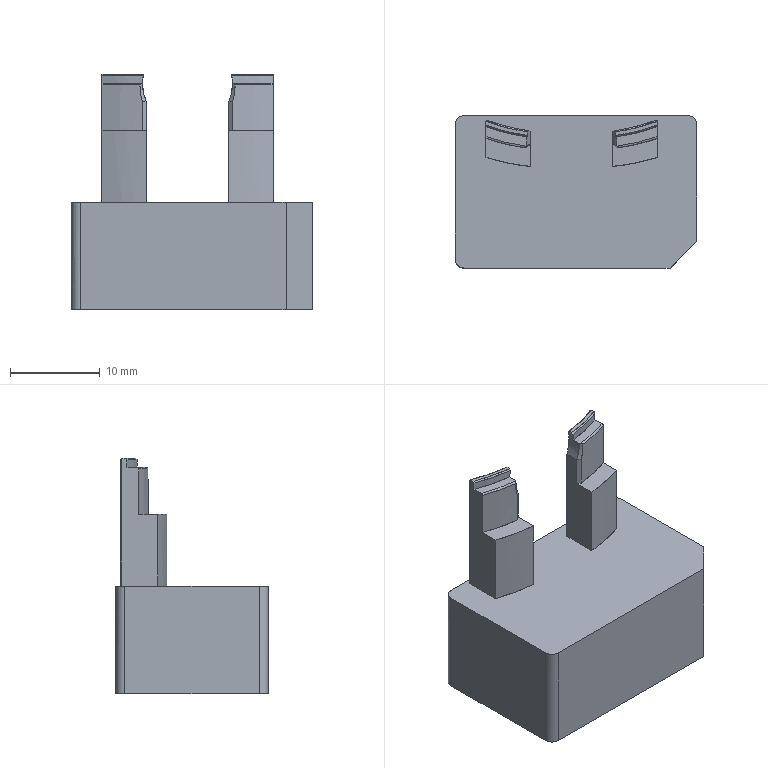NC program | PowerMill | posted by the shop | part box 27 x 17 x 26.255 mm
Lines 16162 to 17310 of 169183:
( TOOL ID   D10_1_1_1 )
( TOOL DIA. 10. TIP RAD 0 LENGTH 81.4 )
( Z = -6.52 )
T3 M6
T10
G91 G28 Z0
G0 G90 G54
M08
S8500 M3
X0 Y0 M8
G43 Z11.805 H3
X-20.807 Y4.302
Z-5.32
G1 Z-6.52 F360
X-15.532 F600
X-15.121 Y4.141
G0 Z4.975
G1 X19.807 Y5.165 F10000
G0 Z-5.32
G1 Z-6.52 F360
X14.532 F600
G3 X14.309 Y4.802 I.367 J-.475
G1 X14.233 Y4.495
X14.146 Y4.213
X14.108 Y4.104
X14.019 Y3.877
X13.918 Y3.649
X13.775 Y3.367
X13.609 Y3.085
X13.467 Y2.869
X13.308 Y2.653
X13.202 Y2.521
X12.988 Y2.276
X12.828 Y2.114
X12.664 Y1.957
X12.423 Y1.751
X12.181 Y1.568
X11.921 Y1.393
X11.618 Y1.215
X11.336 Y1.073
X11.054 Y.95
X10.772 Y.846
X9.927 Y.572
G2 X8.8 Y.25 I-9.077 J29.697
G1 X8.236 Y.109
X7.672 Y-.019
X7.109 Y-.137
X6.545 Y-.242
X5.981 Y-.335
X5.418 Y-.418
X5.136 Y-.454
X4.854 Y-.479
X4.572 Y-.488
X4.291 Y-.483
X4.009 Y-.463
X3.727 Y-.428
X3.445 Y-.378
X3.117 Y-.299
X2.859 Y-.222
X2.6 Y-.13
X2.318 Y-.013
X2.036 Y.125
X1.754 Y.283
X1.473 Y.465
X1.235 Y.639
X.627 Y1.129
X.339 Y1.393
X.072 Y1.675
X-.036 Y1.806
G3 X-.964 Y1.806 I-.463 J-.381
G1 X-1.071 Y1.675
X-1.339 Y1.393
X-1.627 Y1.129
X-2.235 Y.639
X-2.473 Y.465
X-2.786 Y.265
X-3.036 Y.125
X-3.318 Y-.013
X-3.6 Y-.13
X-3.859 Y-.222
X-4.117 Y-.299
X-4.445 Y-.378
X-4.727 Y-.428
X-5.009 Y-.463
X-5.291 Y-.483
X-5.572 Y-.488
X-5.854 Y-.479
X-6.136 Y-.454
X-6.418 Y-.418
X-6.981 Y-.335
X-7.545 Y-.242
X-8.109 Y-.137
X-8.672 Y-.019
X-9.236 Y.109
X-9.854 Y.265
X-10.363 Y.404
X-10.927 Y.572
X-11.772 Y.846
X-12.054 Y.95
X-12.336 Y1.073
X-12.618 Y1.215
X-12.921 Y1.393
X-13.181 Y1.568
X-13.423 Y1.751
X-13.664 Y1.957
X-13.745 Y2.031
X-13.988 Y2.276
X-14.202 Y2.521
X-14.308 Y2.653
X-14.467 Y2.869
X-14.609 Y3.085
X-14.749 Y3.32
X-14.918 Y3.649
X-15.019 Y3.877
X-15.108 Y4.104
X-15.146 Y4.213
X-15.233 Y4.495
X-15.304 Y4.777
X-15.367 Y5.11
X-15.398 Y5.341
X-15.42 Y5.585
G3 X-15.532 Y5.891 I-.598 J-.045
G0 Z3.
G1 X-20.642 Y4.244 F10000
G0 Z-.07
G1 Z-1.27 F360
X-15.439 Y5.113 F600
X-14.935 Y5.009
X-14.872 Y4.874
X-14.823 Y4.777
X-14.665 Y4.495
X-14.483 Y4.213
X-14.308 Y3.973
X-14.178 Y3.811
X-14.037 Y3.649
X-13.896 Y3.5
X-13.745 Y3.352
X-13.595 Y3.215
X-13.44 Y3.085
X-13.181 Y2.887
X-12.899 Y2.699
X-12.591 Y2.521
X-12.323 Y2.386
X-12.054 Y2.27
X-11.49 Y2.064
X-11.176 Y1.957
X-10.77 Y1.826
X-10.363 Y1.699
X-9.8 Y1.538
X-9.236 Y1.389
X-8.672 Y1.254
X-8.109 Y1.131
X-7.545 Y1.021
X-6.981 Y.923
X-6.356 Y.829
X-5.854 Y.77
X-5.572 Y.756
X-5.291 Y.757
X-5.009 Y.773
X-4.727 Y.804
X-4.566 Y.829
X-4.364 Y.867
X-4.163 Y.912
X-3.882 Y.989
X-3.6 Y1.084
X-3.318 Y1.196
X-3.036 Y1.328
X-2.911 Y1.393
X-2.692 Y1.517
X-2.473 Y1.655
X-2.268 Y1.799
X-2.063 Y1.957
X-1.909 Y2.086
X-1.692 Y2.287
X-.963 Y2.137
X-.753 Y2.479
X-.693 Y2.589
X-.58 Y2.811
X-.5 Y2.99
X-.417 Y2.806
X-.306 Y2.586
X-.243 Y2.471
X-.059 Y2.171
X.078 Y1.971
X.269 Y1.72
X.444 Y1.516
X.624 Y1.324
X.843 Y1.114
X1.123 Y.87
X1.364 Y.679
X1.545 Y.549
X1.688 Y.454
X2.076 Y.227
X2.332 Y.099
X2.648 Y-.037
X2.811 Y-.098
X2.976 Y-.154
X3.298 Y-.247
X3.62 Y-.318
X3.942 Y-.37
X4.264 Y-.403
X4.586 Y-.416
X4.908 Y-.41
X5.229 Y-.385
X5.548 Y-.344
X6.182 Y-.248
X6.817 Y-.137
X7.451 Y-.011
X8.085 Y.131
X8.41 Y.21
X5.382 Y.832
X5.981 Y.923
X6.545 Y1.021
X7.109 Y1.131
X7.672 Y1.254
X8.236 Y1.389
X8.8 Y1.538
X9.363 Y1.699
X9.927 Y1.875
X10.49 Y2.064
X11.054 Y2.27
X11.323 Y2.386
X11.618 Y2.535
X11.899 Y2.699
X12.181 Y2.887
X12.272 Y2.956
X13.366 Y2.731
X15.473 Y2.298
G3 X18.256 Y2.838 I.742 J3.611
G1 X20.422 Y4.277
G3 X19.806 Y6.321 I-.617 J.929
G1 X14.531 Y6.327
G3 X14.272 Y5.966 I.324 J-.505
G2 X14.077 Y5.341 I-4.97 J1.213
G1 X13.912 Y4.957
X13.823 Y4.777
X13.665 Y4.495
X13.483 Y4.213
X13.308 Y3.973
X13.244 Y3.892
X13.037 Y3.649
X12.896 Y3.5
X12.745 Y3.352
X12.44 Y3.085
X12.181 Y2.887
X11.899 Y2.699
X11.591 Y2.521
X11.323 Y2.386
X11.054 Y2.27
X10.49 Y2.064
X9.927 Y1.875
X9.363 Y1.699
X8.8 Y1.538
X8.236 Y1.389
X7.672 Y1.254
X7.109 Y1.131
X6.545 Y1.021
X5.981 Y.923
X5.356 Y.829
X4.854 Y.77
X4.572 Y.756
X4.291 Y.757
X4.009 Y.773
X3.727 Y.804
X3.445 Y.85
X3.163 Y.912
X2.882 Y.989
X2.562 Y1.099
X2.318 Y1.196
X2.036 Y1.328
X1.863 Y1.42
X1.692 Y1.517
G2 X1.268 Y1.799 I3.12 J5.164
G1 X1.063 Y1.957
X.909 Y2.086
X.688 Y2.291
X.466 Y2.521
X.345 Y2.659
X.196 Y2.844
X.02 Y3.085
X.001 Y3.114
G3 X-1.003 Y3.111 I-.501 J-.33
G1 X-1.059 Y3.029
X-1.196 Y2.844
X-1.345 Y2.659
X-1.466 Y2.521
X-1.688 Y2.291
X-1.909 Y2.086
X-2.063 Y1.957
X-2.268 Y1.799
X-2.473 Y1.655
X-2.692 Y1.517
X-2.911 Y1.393
X-3.036 Y1.328
X-3.318 Y1.196
X-3.6 Y1.084
X-3.882 Y.989
X-4.163 Y.912
X-4.364 Y.867
X-4.566 Y.829
X-4.727 Y.804
X-5.009 Y.773
X-5.291 Y.757
X-5.572 Y.756
X-5.854 Y.77
X-6.418 Y.837
X-6.981 Y.923
X-7.545 Y1.021
X-8.109 Y1.131
X-8.672 Y1.254
X-9.236 Y1.389
X-9.8 Y1.538
X-10.363 Y1.699
X-10.77 Y1.826
X-11.176 Y1.957
X-11.49 Y2.064
X-12.054 Y2.27
X-12.323 Y2.386
X-12.618 Y2.535
X-12.899 Y2.699
X-13.181 Y2.887
X-13.44 Y3.085
X-13.595 Y3.215
X-13.745 Y3.352
X-13.896 Y3.5
X-14.037 Y3.649
X-14.178 Y3.811
X-14.308 Y3.973
X-14.483 Y4.213
X-14.665 Y4.495
X-14.823 Y4.777
X-14.912 Y4.957
X-15.077 Y5.341
G2 X-15.275 Y5.974 I4.87 J1.87
G3 X-15.532 Y6.334 I-.582 J-.144
G0 Z4.005
G1 X-20.527 Y4.987 F10000
G0 Z.935
G1 Z-.265 F360
X-15.403 Y6.242 F600
X-.606 Y3.671
X-.558 Y3.76
X-.5 Y3.878
X-.435 Y3.745
X-.37 Y3.63
X9.758 Y1.87
X10.308 Y2.05
X10.944 Y2.277
X11.266 Y2.407
X11.589 Y2.562
X11.94 Y2.762
X12.227 Y2.953
X12.393 Y3.076
X12.554 Y3.204
X12.782 Y3.405
X12.876 Y3.494
X13.101 Y3.727
X13.197 Y3.835
X13.374 Y4.05
X13.519 Y4.245
X13.608 Y4.374
X13.841 Y4.756
X13.943 Y4.952
X-15.097 Y9.999
X-15.025 Y10.162
X-14.864 Y10.482
X-14.786 Y10.619
X-14.673 Y10.805
X-14.463 Y11.111
X-14.194 Y11.447
X-14.141 Y11.508
X-13.892 Y11.769
X-13.819 Y11.84
X-13.531 Y12.093
X-13.174 Y12.363
X-12.852 Y12.57
X-12.551 Y12.736
X-12.208 Y12.897
X-11.886 Y13.023
X-11.564 Y13.127
X-11.406 Y13.167
X-3.358 Y11.768
X-3.277 Y11.735
X-2.956 Y11.586
X-2.735 Y11.468
X-2.633 Y11.409
X-2.314 Y11.204
X-2.229 Y11.145
X-1.991 Y10.964
X-1.823 Y10.823
X-1.669 Y10.684
X-1.484 Y10.501
X-1.347 Y10.354
X-1.196 Y10.178
X-1.028 Y9.964
X-.943 Y9.847
X-.738 Y9.533
X-.561 Y9.218
X-.499 Y9.093
X-.44 Y9.217
X-.258 Y9.539
X-.048 Y9.86
X.08 Y10.033
X.199 Y10.182
X.402 Y10.414
X.487 Y10.504
X.724 Y10.735
X.826 Y10.826
X1.041 Y11.004
X14.47 Y8.67
G0 Z11.805
X0 Y0
Z9.805
X-10.046 Y19.255
Z-13.25
G1 Z-14.45 F360
Y13.98 F600
X-10.041 Y13.349
X-9.865 Y13.35
X-9.606 Y13.34
X-9.301 Y13.312
X-9.019 Y13.271
X-8.737 Y13.214
X-8.455 Y13.143
X-8.174 Y13.054
X-7.61 Y12.854
X-7.297 Y12.75
X-7.064 Y12.68
X-6.482 Y12.52
X-5.919 Y12.387
X-5.355 Y12.274
X-3.946 Y12.011
X-3.664 Y11.94
X-3.382 Y11.853
X-3.1 Y11.748
X-2.801 Y11.617
X-2.537 Y11.483
X-2.255 Y11.318
X-1.973 Y11.129
X-1.792 Y10.993
X-1.601 Y10.836
X-1.409 Y10.663
X-1.229 Y10.484
G3 X.229 Y10.484 I.729 J.685
G1 X.282 Y10.538
X.564 Y10.804
X.866 Y11.05
X1.138 Y11.242
X1.409 Y11.411
X1.691 Y11.564
X1.973 Y11.695
X2.255 Y11.808
X2.537 Y11.903
X2.818 Y11.981
X3.1 Y12.042
X4.228 Y12.251
X4.791 Y12.36
X5.355 Y12.487
X5.919 Y12.638
X6.297 Y12.75
X6.482 Y12.811
X7.328 Y13.105
X7.61 Y13.184
X7.892 Y13.247
X8.174 Y13.295
X8.346 Y13.317
X8.737 Y13.346
X9.019 Y13.35
X9.301 Y13.34
X9.583 Y13.315
X9.865 Y13.274
X10.146 Y13.219
X10.428 Y13.148
X10.71 Y13.061
X10.992 Y12.957
X11.219 Y12.86
X11.446 Y12.75
X11.556 Y12.693
X11.838 Y12.529
X12.119 Y12.342
X12.332 Y12.184
X12.464 Y12.078
X12.683 Y11.884
X12.951 Y11.617
X13.127 Y11.419
X13.247 Y11.273
X13.414 Y11.05
X13.604 Y10.767
X13.769 Y10.484
X13.94 Y10.14
X14.036 Y9.917
X14.141 Y9.634
X14.228 Y9.35
X14.3 Y9.067
X14.355 Y8.784
X14.374 Y8.662
X14.421 Y8.217
X14.432 Y7.934
X14.43 Y3.683
X14.414 Y3.4
X14.374 Y3.053
X14.332 Y2.804
X14.275 Y2.55
X14.197 Y2.267
X14.102 Y1.983
X13.989 Y1.7
X13.856 Y1.417
X13.811 Y1.328
X13.677 Y1.09
X13.526 Y.85
X13.393 Y.66
X13.247 Y.47
X13.09 Y.283
X12.898 Y.076
X12.683 Y-.131
X12.509 Y-.283
X12.314 Y-.439
X12.119 Y-.581
X11.904 Y-.723
X11.69 Y-.85
X11.556 Y-.923
X11.274 Y-1.061
X11.182 Y-1.1
X13.146 Y-5.488
G2 X13.768 Y-6.125 I.194 J-.433
G1 X13.764 Y-6.134
G2 X13.658 Y-6.278 I-.429 J.204
G1 X11.513 Y-8.27
G2 X10.898 Y-8.66 I-1.361 J1.466
G1 X10.329 Y-8.888
G2 X9.581 Y-9.032 I-.745 J1.856
G1 X-11.982 Y-9.007
G2 X-12.928 Y-8.764 I.002 J1.973
G1 X-13.284 Y-8.569
G2 X-14.102 Y-7.365 I.769 J1.402
G1 X-14.159 Y-6.91
G2 X-12.877 Y-5.957 I.911 J.114
G1 X-12.543 Y-6.104
G3 X-3.23 Y-7.175 I6.375 J14.419
G1 X-.871 Y-6.728
G2 X-.118 Y-6.729 I.373 J-1.965
G1 X2.479 Y-7.232
G3 X11.592 Y-6.183 I2.896 J14.941
G1 X13.146 Y-5.488
X11.182 Y-1.1
X10.992 Y-1.18
X10.71 Y-1.28
X9.865 Y-1.532
X9.301 Y-1.686
X8.737 Y-1.827
X8.174 Y-1.958
X7.61 Y-2.076
X7.046 Y-2.184
X6.482 Y-2.281
X5.919 Y-2.367
X5.355 Y-2.443
X4.791 Y-2.509
X4.52 Y-2.537
X4.228 Y-2.551
X3.971 Y-2.55
X3.664 Y-2.533
X3.382 Y-2.502
X3.1 Y-2.457
X2.818 Y-2.395
X2.537 Y-2.317
X2.255 Y-2.222
X1.973 Y-2.109
X1.703 Y-1.983
X1.409 Y-1.825
X1.127 Y-1.65
X.804 Y-1.417
X.543 Y-1.2
X.282 Y-.952
X.22 Y-.888
G3 X-1.21 Y-.877 I-.721 J-.693
G1 X-1.409 Y-1.077
X-1.607 Y-1.256
X-1.804 Y-1.417
X-1.973 Y-1.543
X-2.255 Y-1.732
X-2.537 Y-1.897
X-2.703 Y-1.983
X-3.1 Y-2.163
X-3.382 Y-2.267
X-3.664 Y-2.354
X-3.946 Y-2.424
X-4.228 Y-2.479
X-4.51 Y-2.518
X-4.791 Y-2.543
X-4.971 Y-2.55
X-5.249
X-5.355 Y-2.546
X-5.637 Y-2.526
X-6.482 Y-2.427
X-7.046 Y-2.348
X-7.61 Y-2.26
X-8.174 Y-2.16
X-8.737 Y-2.05
X-9.301 Y-1.929
X-9.865 Y-1.796
X-10.428 Y-1.652
X-10.992 Y-1.496
X-11.416 Y-1.37
X-11.838 Y-1.236
X-12.119 Y-1.128
X-12.401 Y-1.002
X-12.683 Y-.854
X-12.969 Y-.682
X-13.247 Y-.49
X-13.509 Y-.283
X-13.663 Y-.15
X-13.811 Y-.011
X-13.956 Y.136
X-14.09 Y.283
X-14.238 Y.459
X-14.374 Y.635
X-14.526 Y.85
X-14.702 Y1.133
X-14.856 Y1.417
X-14.938 Y1.587
X-15.102 Y1.983
X-15.197 Y2.267
X-15.275 Y2.55
X-15.337 Y2.833
X-15.383 Y3.117
X-15.414 Y3.4
X-15.43 Y3.683
X-15.432 Y7.934
X-15.421 Y8.217
X-15.395 Y8.5
X-15.355 Y8.784
X-15.3 Y9.067
X-15.228 Y9.35
X-15.141 Y9.634
X-15.036 Y9.917
X-14.938 Y10.144
X-14.769 Y10.484
X-14.604 Y10.767
X-14.374 Y11.105
X-14.196 Y11.337
X-13.951 Y11.617
X-13.811 Y11.762
X-13.529 Y12.023
X-13.332 Y12.184
X-13.247 Y12.249
X-12.964 Y12.448
X-12.683 Y12.621
X-12.446 Y12.75
X-12.119 Y12.904
X-11.838 Y13.016
X-11.556 Y13.111
X-11.274 Y13.188
X-10.992 Y13.251
X-10.71 Y13.298
X-10.428 Y13.33
X-10.146 Y13.348
X-10.041 Y13.349
X-10.046 Y13.98
G0 Z9.805
X0 Y0
X18.473 Y-14.782
Z-25.15
G1 Z-26.35 F360
G3 X14.938 Y-11.246 I-1.768 J1.768 F600
G1 X14.114 Y-12.07
Y-12.071
X14.113
X13.966 Y-12.214
X13.965 Y-12.215
X13.963 Y-12.216
X13.768 Y-12.39
X13.766 Y-12.391
X13.765 Y-12.392
X13.645 Y-12.49
X13.643 Y-12.491
X13.641 Y-12.492
X13.342 Y-12.71
X13.34 Y-12.712
X13.337 Y-12.714
X13.004 Y-12.92
X13.002 Y-12.921
X13. Y-12.922
X12.794 Y-13.033
X12.793
X12.792 Y-13.034
X12.681 Y-13.088
X12.679 Y-13.089
X12.678 Y-13.09
X12.362 Y-13.227
X12.359 Y-13.228
X12.356 Y-13.229
X11.999 Y-13.354
X11.997
X11.994 Y-13.355
X11.719 Y-13.432
X11.716
X11.714 Y-13.433
X11.398 Y-13.5
X11.395
X11.393 Y-13.501
X11.077 Y-13.547
X11.074
X11.072 Y-13.548
X10.755 Y-13.574
X10.753
X10.751
X10.434 Y-13.58
X10.433
X-12.33
X-12.646 Y-13.578
X-12.648
X-12.65
X-12.966 Y-13.562
X-12.968
X-12.97
X-13.286 Y-13.529
X-13.289
X-13.291 Y-13.528
X-13.607 Y-13.478
X-13.609
X-13.611
X-13.927 Y-13.41
X-13.929
X-13.931 Y-13.409
X-14.247 Y-13.323
X-14.25
X-14.252 Y-13.322
X-14.568 Y-13.217
X-14.57 Y-13.216
X-14.572
X-14.888 Y-13.091
X-14.89
X-14.891 Y-13.09
X-15.016 Y-13.035
X-15.017
X-15.018 Y-13.034
X-15.21 Y-12.942
X-15.211
X-15.213 Y-12.941
X-15.529 Y-12.772
X-15.531 Y-12.771
X-15.533 Y-12.769
X-15.849 Y-12.574
X-15.851 Y-12.573
X-15.854 Y-12.571
X-16.17 Y-12.348
X-16.172 Y-12.346
X-16.174 Y-12.344
X-16.49 Y-12.088
X-16.492 Y-12.086
X-16.494 Y-12.084
X-16.81 Y-11.788
X-16.813 Y-11.786
X-16.815 Y-11.784
X-17.131 Y-11.439
X-17.133 Y-11.437
X-17.134 Y-11.435
X-17.389 Y-11.115
X-17.39 Y-11.113
X-17.392 Y-11.111
X-17.61 Y-10.794
X-17.611 Y-10.792
X-17.612 Y-10.791
X-17.772 Y-10.528
X-17.774 Y-10.526
X-17.775 Y-10.523
X-17.97 Y-10.154
X-17.971 Y-10.152
X-17.972 Y-10.15
X-18.093 Y-9.884
X-18.094 Y-9.882
X-18.095 Y-9.88
X-18.237 Y-9.513
X-18.238 Y-9.511
X-18.239 Y-9.509
X-18.34 Y-9.193
Y-9.191
X-18.341 Y-9.189
X-18.414 Y-8.912
Y-8.91
X-18.415 Y-8.907
X-18.488 Y-8.552
Y-8.55
Y-8.548
X-18.536 Y-8.232
Y-8.229
Y-8.227
X-18.565 Y-7.911
Y-7.909
X-18.566 Y-7.907
X-18.579 Y-7.591
Y-7.589
Y-7.587
Y7.587
Y7.589
Y7.591
X-18.566 Y7.907
Y7.909
Y7.911
X-18.536 Y8.227
Y8.229
Y8.231
X-18.489 Y8.548
Y8.55
X-18.488 Y8.552
X-18.424 Y8.868
Y8.87
X-18.423 Y8.872
X-18.341 Y9.188
X-18.34 Y9.19
Y9.193
X-18.238 Y9.509
Y9.511
X-18.237 Y9.513
X-18.116 Y9.829
X-18.115 Y9.831
X-18.114 Y9.833
X-17.972 Y10.149
X-17.971 Y10.152
X-17.97 Y10.154
X-17.805 Y10.47
X-17.804 Y10.472
X-17.803 Y10.474
X-17.613 Y10.79
X-17.611 Y10.792
X-17.61 Y10.794
X-17.454 Y11.024
Y11.025
X-17.453 Y11.027
X-17.391 Y11.112
X-17.39 Y11.113
X-17.389 Y11.115
X-17.138 Y11.431
X-17.137 Y11.433
X-17.135 Y11.435
X-16.846 Y11.751
X-16.844 Y11.753
X-16.842 Y11.756
X-16.508 Y12.072
X-16.506 Y12.074
X-16.504 Y12.076
X-16.174 Y12.344
X-16.172 Y12.346
X-16.17 Y12.348
X-15.853 Y12.571
X-15.852 Y12.572
X-15.85 Y12.573
X-15.628 Y12.713
X-15.627 Y12.714
X-15.626 Y12.715
X-15.532 Y12.77
X-15.53 Y12.771
X-15.529 Y12.772
X-15.213 Y12.941
X-15.211 Y12.942
X-15.209 Y12.943
X-14.892 Y13.089
X-14.89 Y13.09
X-14.888 Y13.091
X-14.572 Y13.216
X-14.57 Y13.217
X-14.568 Y13.218
X-14.252 Y13.322
X-14.25 Y13.323
X-14.247
X-13.931 Y13.409
X-13.929 Y13.41
X-13.927
X-13.611 Y13.477
X-13.609 Y13.478
X-13.607
X-13.291 Y13.528
X-13.288 Y13.529
X-13.286
X-12.97 Y13.561
X-12.968 Y13.562
X-12.966
X-12.65 Y13.578
X-12.648
X-12.646
X-12.33 Y13.58
X0
X12.33
X12.646 Y13.578
X12.648
X12.65
X12.966 Y13.562
X12.968
X12.97
X13.286 Y13.529
X13.289
X13.291 Y13.528
X13.607 Y13.478
X13.609
X13.611
X13.927 Y13.41
X13.929
X13.931 Y13.409
X14.247 Y13.323
X14.25
X14.252 Y13.322
X14.568 Y13.217
X14.57 Y13.216
X14.572
X14.888 Y13.091
X14.89
X14.891 Y13.09
X15.016 Y13.035
X15.017
X15.018 Y13.034
X15.21 Y12.942
X15.211
X15.213 Y12.941
X15.529 Y12.772
X15.531 Y12.771
X15.533 Y12.769
X15.849 Y12.574
X15.851 Y12.573
X15.854 Y12.571
X16.17 Y12.348
X16.172 Y12.346
X16.174 Y12.344
X16.49 Y12.088
X16.492 Y12.086
X16.494 Y12.084
X16.81 Y11.788
X16.813 Y11.786
X16.815 Y11.784
X17.131 Y11.439
X17.133 Y11.437
X17.135 Y11.435
X17.389 Y11.115
X17.39 Y11.113
X17.391 Y11.112
X17.453 Y11.026
X17.454 Y11.025
Y11.024
X17.61 Y10.794
X17.611 Y10.792
X17.612 Y10.791
X17.772 Y10.528
X17.774 Y10.526
X17.775 Y10.523
X17.97 Y10.154
X17.971 Y10.152
X17.972 Y10.15
X18.093 Y9.884
X18.094 Y9.882
X18.095 Y9.88
X18.237 Y9.513
X18.238 Y9.511
X18.239 Y9.509
X18.34 Y9.193
Y9.191
X18.341 Y9.189
X18.414 Y8.912
Y8.91
X18.415 Y8.907
X18.488 Y8.552
Y8.55
Y8.548
X18.536 Y8.232
Y8.229
Y8.227
X18.565 Y7.911
Y7.909
X18.566 Y7.907
X18.579 Y7.591
Y7.589
Y7.588
X18.58 Y-5.374
Y-5.375
X18.576 Y-5.692
Y-5.694
Y-5.696
X18.554 Y-6.012
Y-6.015
Y-6.017
X18.511 Y-6.334
Y-6.336
X18.51 Y-6.339
X18.447 Y-6.655
Y-6.657
X18.446 Y-6.658
X18.414 Y-6.788
Y-6.789
X18.413 Y-6.79
X18.361 Y-6.977
X18.36 Y-6.979
X18.359 Y-6.981
X18.251 Y-7.297
Y-7.3
X18.25 Y-7.302
X18.117 Y-7.618
X18.116 Y-7.621
X18.115 Y-7.623
X17.956 Y-7.94
X17.955 Y-7.942
X17.953 Y-7.945
X17.773 Y-8.247
X17.771 Y-8.25
X17.77 Y-8.252
X17.538 Y-8.582
X17.537 Y-8.584
X17.536 Y-8.585
X17.451 Y-8.693
X17.45 Y-8.695
X17.449 Y-8.696
X17.271 Y-8.904
X17.269 Y-8.905
X17.268 Y-8.907
X17.13 Y-9.054
X17.129 Y-9.055
X17.128
X14.938 Y-11.246
G3 X18.473 Y-14.782 I1.768 J-1.768
G1 X18.422 Y-14.72
G3 X14.886 Y-11.185 I-1.768 J1.768
G1 X14.058 Y-12.014
X13.91 Y-12.156
X13.715 Y-12.33
X13.594 Y-12.428
X13.295 Y-12.646
X12.962 Y-12.852
X12.756 Y-12.962
X12.646 Y-13.016
X12.33 Y-13.153
X11.973 Y-13.278
X11.697 Y-13.355
X11.381 Y-13.422
X11.065 Y-13.468
X10.749 Y-13.494
X10.433 Y-13.5
X-12.33
X-12.646 Y-13.498
X-12.962 Y-13.482
X-13.278 Y-13.449
X-13.594 Y-13.399
X-13.91 Y-13.332
X-14.227 Y-13.246
X-14.543 Y-13.141
X-14.859 Y-13.017
X-14.983 Y-12.962
X-15.175 Y-12.87
X-15.491 Y-12.701
X-15.807 Y-12.506
X-16.123 Y-12.282
X-16.44 Y-12.025
X-16.756 Y-11.73
X-17.072 Y-11.385
X-17.326 Y-11.065
X-17.544 Y-10.749
X-17.704 Y-10.486
X-17.899 Y-10.117
X-18.02 Y-9.851
X-18.162 Y-9.484
X-18.263 Y-9.168
X-18.336 Y-8.891
X-18.409 Y-8.536
X-18.457 Y-8.22
X-18.486 Y-7.904
X-18.499 Y-7.587
X-18.5 Y-7.271
Y7.271
X-18.499 Y7.587
X-18.486 Y7.904
X-18.457 Y8.22
X-18.41 Y8.536
X-18.346 Y8.852
X-18.263 Y9.168
X-18.162 Y9.484
X-18.041 Y9.801
X-17.899 Y10.117
X-17.734 Y10.433
X-17.544 Y10.749
X-17.388 Y10.98
X-17.326 Y11.065
X-17.076 Y11.381
X-16.787 Y11.697
X-16.453 Y12.014
X-16.123 Y12.282
X-15.807 Y12.505
X-15.585 Y12.646
X-15.491 Y12.701
X-15.175 Y12.871
X-14.859 Y13.017
X-14.543 Y13.142
X-14.227 Y13.246
X-13.91 Y13.332
X-13.594 Y13.399
X-13.278 Y13.449
X-12.962 Y13.482
X-12.646 Y13.498
X-12.33 Y13.5
X0
X12.33
X12.646 Y13.498
X12.962 Y13.482
X13.278 Y13.449
X13.594 Y13.399
X13.91 Y13.332
X14.227 Y13.246
X14.543 Y13.141
X14.859 Y13.017
X14.983 Y12.962
X15.175 Y12.87
X15.491 Y12.701
X15.807 Y12.506
X16.123 Y12.282
X16.44 Y12.025
X16.756 Y11.73
X17.072 Y11.385
X17.326 Y11.065
X17.388 Y10.979
X17.544 Y10.749
X17.704 Y10.486
X17.899 Y10.117
X18.02 Y9.851
X18.162 Y9.484
X18.263 Y9.168
X18.336 Y8.891
X18.409 Y8.536
X18.457 Y8.22
X18.486 Y7.904
X18.499 Y7.587
X18.5 Y7.271
Y-5.374
X18.496 Y-5.691
X18.474 Y-6.007
X18.432 Y-6.323
X18.369 Y-6.639
X18.336 Y-6.768
X18.284 Y-6.955
X18.176 Y-7.271
X18.043 Y-7.587
X17.884 Y-7.904
X17.704 Y-8.206
X17.473 Y-8.536
X17.388 Y-8.644
X17.21 Y-8.852
X17.072 Y-8.999
X14.886 Y-11.185
G3 X18.422 Y-14.72 I1.768 J-1.768
G0 Z9.805
Z10.805
X0 Y0
M9
M5
M01